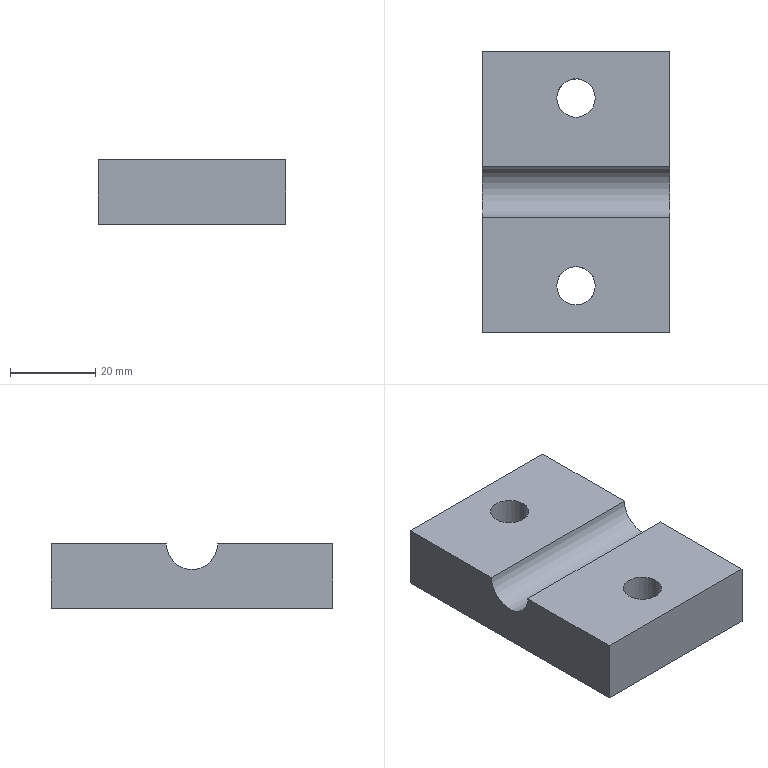Part | 1 solid | 12 faces | box 44 x 66 x 15 mm | volume 39164 mm3 | plane 7 | cylinder 5 | commonest cylinder face diameters 9 x4 12 x1
STEP:
#1=CARTESIAN_POINT('',(0.,0.,0.));
#2=DIRECTION('',(0.,0.,1.));
#3=DIRECTION('',(1.,0.,0.));
#4=AXIS2_PLACEMENT_3D('',#1,#2,#3);
#5=CARTESIAN_POINT('',(-482.433,147.5,-310.6));
#6=VERTEX_POINT('',#5);
#7=CARTESIAN_POINT('',(-526.433,147.5,-310.6));
#8=VERTEX_POINT('',#7);
#9=CARTESIAN_POINT('',(-517.416,147.5,-310.6));
#10=DIRECTION('',(-1.,0.,0.));
#11=VECTOR('',#10,1.);
#12=LINE('',#9,#11);
#13=CARTESIAN_POINT('',(-504.433,141.5,-310.6));
#14=DIRECTION('',(0.,0.,1.));
#15=DIRECTION('',(-1.,0.,0.));
#16=AXIS2_PLACEMENT_3D('',#13,#14,#15);
#17=PLANE('',#16);
#18=CARTESIAN_POINT('',(12.983,-6.));
#19=DIRECTION('',(1.,0.));
#20=VECTOR('',#19,1.);
#21=LINE('',#18,#20);
#22=(GEOMETRIC_REPRESENTATION_CONTEXT(2)PARAMETRIC_REPRESENTATION_CONTEXT()REPRESENTATION_CONTEXT('',''));
#23=DEFINITIONAL_REPRESENTATION('',(#21),#22);
#24=PCURVE('',#17,#23);
#25=CARTESIAN_POINT('',(-517.416,141.5,-310.6));
#26=DIRECTION('',(-1.,0.,0.));
#27=DIRECTION('',(0.,0.,1.));
#28=AXIS2_PLACEMENT_3D('',#25,#26,#27);
#29=CYLINDRICAL_SURFACE('',#28,6.);
#30=CARTESIAN_POINT('',(1.571,0.));
#31=DIRECTION('',(0.,1.));
#32=VECTOR('',#31,1.);
#33=LINE('',#30,#32);
#34=(GEOMETRIC_REPRESENTATION_CONTEXT(2)PARAMETRIC_REPRESENTATION_CONTEXT()REPRESENTATION_CONTEXT('',''));
#35=DEFINITIONAL_REPRESENTATION('',(#33),#34);
#36=PCURVE('',#29,#35);
#37=SURFACE_CURVE('',#12,(#24,#36),.PCURVE_S1.);
#38=EDGE_CURVE('',#6,#8,#37,.T.);
#39=ORIENTED_EDGE('',*,*,#38,.F.);
#40=CARTESIAN_POINT('',(-482.433,174.5,-310.6));
#41=VERTEX_POINT('',#40);
#42=CARTESIAN_POINT('',(-482.433,141.5,-310.6));
#43=DIRECTION('',(0.,-1.,0.));
#44=VECTOR('',#43,1.);
#45=LINE('',#42,#44);
#46=CARTESIAN_POINT('',(-22.,0.));
#47=DIRECTION('',(0.,1.));
#48=VECTOR('',#47,1.);
#49=LINE('',#46,#48);
#50=(GEOMETRIC_REPRESENTATION_CONTEXT(2)PARAMETRIC_REPRESENTATION_CONTEXT()REPRESENTATION_CONTEXT('',''));
#51=DEFINITIONAL_REPRESENTATION('',(#49),#50);
#52=PCURVE('',#17,#51);
#53=CARTESIAN_POINT('',(-482.433,141.5,-319.1));
#54=DIRECTION('',(1.,0.,0.));
#55=DIRECTION('',(0.,0.,1.));
#56=AXIS2_PLACEMENT_3D('',#53,#54,#55);
#57=PLANE('',#56);
#58=CARTESIAN_POINT('',(8.5,0.));
#59=DIRECTION('',(0.,1.));
#60=VECTOR('',#59,1.);
#61=LINE('',#58,#60);
#62=(GEOMETRIC_REPRESENTATION_CONTEXT(2)PARAMETRIC_REPRESENTATION_CONTEXT()REPRESENTATION_CONTEXT('',''));
#63=DEFINITIONAL_REPRESENTATION('',(#61),#62);
#64=PCURVE('',#57,#63);
#65=SURFACE_CURVE('',#45,(#52,#64),.PCURVE_S1.);
#66=EDGE_CURVE('',#41,#6,#65,.T.);
#67=ORIENTED_EDGE('',*,*,#66,.F.);
#68=CARTESIAN_POINT('',(-526.433,174.5,-310.6));
#69=VERTEX_POINT('',#68);
#70=CARTESIAN_POINT('',(-504.433,174.5,-310.6));
#71=DIRECTION('',(1.,0.,0.));
#72=VECTOR('',#71,1.);
#73=LINE('',#70,#72);
#74=CARTESIAN_POINT('',(0.,-33.));
#75=DIRECTION('',(-1.,0.));
#76=VECTOR('',#75,1.);
#77=LINE('',#74,#76);
#78=(GEOMETRIC_REPRESENTATION_CONTEXT(2)PARAMETRIC_REPRESENTATION_CONTEXT()REPRESENTATION_CONTEXT('',''));
#79=DEFINITIONAL_REPRESENTATION('',(#77),#78);
#80=PCURVE('',#17,#79);
#81=CARTESIAN_POINT('',(-504.433,174.5,-319.1));
#82=DIRECTION('',(0.,1.,0.));
#83=DIRECTION('',(0.,0.,-1.));
#84=AXIS2_PLACEMENT_3D('',#81,#82,#83);
#85=PLANE('',#84);
#86=CARTESIAN_POINT('',(-8.5,0.));
#87=DIRECTION('',(0.,-1.));
#88=VECTOR('',#87,1.);
#89=LINE('',#86,#88);
#90=(GEOMETRIC_REPRESENTATION_CONTEXT(2)PARAMETRIC_REPRESENTATION_CONTEXT()REPRESENTATION_CONTEXT('',''));
#91=DEFINITIONAL_REPRESENTATION('',(#89),#90);
#92=PCURVE('',#85,#91);
#93=SURFACE_CURVE('',#73,(#80,#92),.PCURVE_S1.);
#94=EDGE_CURVE('',#69,#41,#93,.T.);
#95=ORIENTED_EDGE('',*,*,#94,.F.);
#96=CARTESIAN_POINT('',(-526.433,141.5,-310.6));
#97=DIRECTION('',(0.,1.,0.));
#98=VECTOR('',#97,1.);
#99=LINE('',#96,#98);
#100=CARTESIAN_POINT('',(22.,0.));
#101=DIRECTION('',(0.,-1.));
#102=VECTOR('',#101,1.);
#103=LINE('',#100,#102);
#104=(GEOMETRIC_REPRESENTATION_CONTEXT(2)PARAMETRIC_REPRESENTATION_CONTEXT()REPRESENTATION_CONTEXT('',''));
#105=DEFINITIONAL_REPRESENTATION('',(#103),#104);
#106=PCURVE('',#17,#105);
#107=CARTESIAN_POINT('',(-526.433,141.5,-319.1));
#108=DIRECTION('',(-1.,0.,0.));
#109=DIRECTION('',(0.,0.,-1.));
#110=AXIS2_PLACEMENT_3D('',#107,#108,#109);
#111=PLANE('',#110);
#112=CARTESIAN_POINT('',(-8.5,0.));
#113=DIRECTION('',(0.,-1.));
#114=VECTOR('',#113,1.);
#115=LINE('',#112,#114);
#116=(GEOMETRIC_REPRESENTATION_CONTEXT(2)PARAMETRIC_REPRESENTATION_CONTEXT()REPRESENTATION_CONTEXT('',''));
#117=DEFINITIONAL_REPRESENTATION('',(#115),#116);
#118=PCURVE('',#111,#117);
#119=SURFACE_CURVE('',#99,(#106,#118),.PCURVE_S1.);
#120=EDGE_CURVE('',#8,#69,#119,.T.);
#121=ORIENTED_EDGE('',*,*,#120,.F.);
#122=EDGE_LOOP('',(#39,#67,#95,#121));
#123=FACE_BOUND('',#122,.T.);
#124=CARTESIAN_POINT('',(-508.933,163.5,-310.6));
#125=VERTEX_POINT('',#124);
#126=CARTESIAN_POINT('',(-499.933,163.5,-310.6));
#127=VERTEX_POINT('',#126);
#128=CARTESIAN_POINT('',(-504.433,163.5,-310.6));
#129=DIRECTION('',(0.,0.,-1.));
#130=DIRECTION('',(-1.,0.,0.));
#131=AXIS2_PLACEMENT_3D('',#128,#129,#130);
#132=CIRCLE('',#131,4.5);
#133=CARTESIAN_POINT('',(4.5,-22.));
#134=CARTESIAN_POINT('',(4.5,-29.794));
#135=CARTESIAN_POINT('',(-2.25,-25.897));
#136=CARTESIAN_POINT('',(-9.,-22.));
#137=CARTESIAN_POINT('',(-2.25,-18.103));
#138=CARTESIAN_POINT('',(4.5,-14.206));
#139=CARTESIAN_POINT('',(4.5,-22.));
#140=(BOUNDED_CURVE()B_SPLINE_CURVE(2,(#133,#134,#135,#136,#137,#138,#139),.UNSPECIFIED.,.T.,.F.)B_SPLINE_CURVE_WITH_KNOTS((1,2,2,2,2,1),(-2.094,0.,2.094,4.189,6.283,8.378),.UNSPECIFIED.)CURVE()GEOMETRIC_REPRESENTATION_ITEM()RATIONAL_B_SPLINE_CURVE((1.,0.5,1.,0.5,1.,0.5,1.))REPRESENTATION_ITEM(''));
#141=(GEOMETRIC_REPRESENTATION_CONTEXT(2)PARAMETRIC_REPRESENTATION_CONTEXT()REPRESENTATION_CONTEXT('',''));
#142=DEFINITIONAL_REPRESENTATION('',(#140),#141);
#143=PCURVE('',#17,#142);
#144=CARTESIAN_POINT('',(-504.433,163.5,-608.599));
#145=DIRECTION('',(0.,0.,1.));
#146=DIRECTION('',(0.,-1.,0.));
#147=AXIS2_PLACEMENT_3D('',#144,#145,#146);
#148=CYLINDRICAL_SURFACE('',#147,4.5);
#149=CARTESIAN_POINT('',(4.712,297.999));
#150=DIRECTION('',(-1.,0.));
#151=VECTOR('',#150,1.);
#152=LINE('',#149,#151);
#153=(GEOMETRIC_REPRESENTATION_CONTEXT(2)PARAMETRIC_REPRESENTATION_CONTEXT()REPRESENTATION_CONTEXT('',''));
#154=DEFINITIONAL_REPRESENTATION('',(#152),#153);
#155=PCURVE('',#148,#154);
#156=SURFACE_CURVE('',#132,(#143,#155),.PCURVE_S1.);
#157=EDGE_CURVE('',#125,#127,#156,.T.);
#158=ORIENTED_EDGE('',*,*,#157,.T.);
#159=CARTESIAN_POINT('',(-504.433,163.5,-310.6));
#160=DIRECTION('',(0.,0.,-1.));
#161=DIRECTION('',(-1.,0.,0.));
#162=AXIS2_PLACEMENT_3D('',#159,#160,#161);
#163=CIRCLE('',#162,4.5);
#164=CARTESIAN_POINT('',(4.5,-22.));
#165=CARTESIAN_POINT('',(4.5,-29.794));
#166=CARTESIAN_POINT('',(-2.25,-25.897));
#167=CARTESIAN_POINT('',(-9.,-22.));
#168=CARTESIAN_POINT('',(-2.25,-18.103));
#169=CARTESIAN_POINT('',(4.5,-14.206));
#170=CARTESIAN_POINT('',(4.5,-22.));
#171=(BOUNDED_CURVE()B_SPLINE_CURVE(2,(#164,#165,#166,#167,#168,#169,#170),.UNSPECIFIED.,.T.,.F.)B_SPLINE_CURVE_WITH_KNOTS((1,2,2,2,2,1),(-2.094,0.,2.094,4.189,6.283,8.378),.UNSPECIFIED.)CURVE()GEOMETRIC_REPRESENTATION_ITEM()RATIONAL_B_SPLINE_CURVE((1.,0.5,1.,0.5,1.,0.5,1.))REPRESENTATION_ITEM(''));
#172=(GEOMETRIC_REPRESENTATION_CONTEXT(2)PARAMETRIC_REPRESENTATION_CONTEXT()REPRESENTATION_CONTEXT('',''));
#173=DEFINITIONAL_REPRESENTATION('',(#171),#172);
#174=PCURVE('',#17,#173);
#175=CARTESIAN_POINT('',(-504.433,163.5,-608.599));
#176=DIRECTION('',(0.,0.,1.));
#177=DIRECTION('',(0.,1.,0.));
#178=AXIS2_PLACEMENT_3D('',#175,#176,#177);
#179=CYLINDRICAL_SURFACE('',#178,4.5);
#180=CARTESIAN_POINT('',(7.854,297.999));
#181=DIRECTION('',(-1.,0.));
#182=VECTOR('',#181,1.);
#183=LINE('',#180,#182);
#184=(GEOMETRIC_REPRESENTATION_CONTEXT(2)PARAMETRIC_REPRESENTATION_CONTEXT()REPRESENTATION_CONTEXT('',''));
#185=DEFINITIONAL_REPRESENTATION('',(#183),#184);
#186=PCURVE('',#179,#185);
#187=SURFACE_CURVE('',#163,(#174,#186),.PCURVE_S1.);
#188=EDGE_CURVE('',#127,#125,#187,.T.);
#189=ORIENTED_EDGE('',*,*,#188,.T.);
#190=EDGE_LOOP('',(#158,#189));
#191=FACE_BOUND('',#190,.T.);
#192=ADVANCED_FACE('',(#123,#191),#17,.T.);
#193=CARTESIAN_POINT('',(-499.933,163.5,-325.6));
#194=VERTEX_POINT('',#193);
#195=CARTESIAN_POINT('',(-508.933,163.5,-325.6));
#196=VERTEX_POINT('',#195);
#197=CARTESIAN_POINT('',(-499.933,163.5,-325.6));
#198=CARTESIAN_POINT('',(-499.933,164.914,-325.6));
#199=CARTESIAN_POINT('',(-500.486,166.328,-325.6));
#200=CARTESIAN_POINT('',(-501.604,167.447,-325.6));
#201=CARTESIAN_POINT('',(-504.433,168.554,-325.6));
#202=CARTESIAN_POINT('',(-507.261,167.446,-325.6));
#203=CARTESIAN_POINT('',(-508.38,166.329,-325.6));
#204=CARTESIAN_POINT('',(-508.933,164.913,-325.6));
#205=CARTESIAN_POINT('',(-508.933,163.5,-325.6));
#206=B_SPLINE_CURVE_WITH_KNOTS('',5,(#197,#198,#199,#200,#201,#202,#203,#204,#205),.UNSPECIFIED.,.F.,.F.,(6,3,6),(3.142,4.712,6.283),.UNSPECIFIED.);
#207=CARTESIAN_POINT('',(-1.571,282.999));
#208=DIRECTION('',(1.,0.));
#209=VECTOR('',#208,1.);
#210=LINE('',#207,#209);
#211=(GEOMETRIC_REPRESENTATION_CONTEXT(2)PARAMETRIC_REPRESENTATION_CONTEXT()REPRESENTATION_CONTEXT('',''));
#212=DEFINITIONAL_REPRESENTATION('',(#210),#211);
#213=PCURVE('',#148,#212);
#214=CARTESIAN_POINT('',(-492.022,-194.5,-325.6));
#215=DIRECTION('',(-0.00001444,0.,-1.));
#216=DIRECTION('',(1.,0.,-0.00001444));
#217=AXIS2_PLACEMENT_3D('',#214,#215,#216);
#218=PLANE('',#217);
#219=CARTESIAN_POINT('',(-7.911,-358.));
#220=CARTESIAN_POINT('',(-7.911,-359.414));
#221=CARTESIAN_POINT('',(-8.464,-360.828));
#222=CARTESIAN_POINT('',(-9.582,-361.946));
#223=CARTESIAN_POINT('',(-12.411,-363.053));
#224=CARTESIAN_POINT('',(-15.239,-361.946));
#225=CARTESIAN_POINT('',(-16.358,-360.829));
#226=CARTESIAN_POINT('',(-16.911,-359.413));
#227=CARTESIAN_POINT('',(-16.911,-358.));
#228=B_SPLINE_CURVE_WITH_KNOTS('',5,(#219,#220,#221,#222,#223,#224,#225,#226,#227),.UNSPECIFIED.,.F.,.F.,(6,3,6),(3.142,4.712,6.283),.UNSPECIFIED.);
#229=(GEOMETRIC_REPRESENTATION_CONTEXT(2)PARAMETRIC_REPRESENTATION_CONTEXT()REPRESENTATION_CONTEXT('',''));
#230=DEFINITIONAL_REPRESENTATION('',(#228),#229);
#231=PCURVE('',#218,#230);
#232=SURFACE_CURVE('',#206,(#213,#231),.PCURVE_S1.);
#233=EDGE_CURVE('',#194,#196,#232,.T.);
#234=ORIENTED_EDGE('',*,*,#233,.T.);
#235=CARTESIAN_POINT('',(-508.933,163.5,-325.6));
#236=DIRECTION('',(0.,0.,1.));
#237=VECTOR('',#236,1.);
#238=LINE('',#235,#237);
#239=CARTESIAN_POINT('',(4.712,282.999));
#240=DIRECTION('',(0.,1.));
#241=VECTOR('',#240,1.);
#242=LINE('',#239,#241);
#243=(GEOMETRIC_REPRESENTATION_CONTEXT(2)PARAMETRIC_REPRESENTATION_CONTEXT()REPRESENTATION_CONTEXT('',''));
#244=DEFINITIONAL_REPRESENTATION('',(#242),#243);
#245=PCURVE('',#148,#244);
#246=CARTESIAN_POINT('',(1.571,282.999));
#247=DIRECTION('',(0.,1.));
#248=VECTOR('',#247,1.);
#249=LINE('',#246,#248);
#250=(GEOMETRIC_REPRESENTATION_CONTEXT(2)PARAMETRIC_REPRESENTATION_CONTEXT()REPRESENTATION_CONTEXT('',''));
#251=DEFINITIONAL_REPRESENTATION('',(#249),#250);
#252=PCURVE('',#179,#251);
#253=SURFACE_CURVE('',#238,(#245,#252),.PCURVE_S1.);
#254=EDGE_CURVE('',#196,#125,#253,.T.);
#255=ORIENTED_EDGE('',*,*,#254,.T.);
#256=ORIENTED_EDGE('',*,*,#157,.T.);
#257=CARTESIAN_POINT('',(-499.933,163.5,-325.6));
#258=DIRECTION('',(0.,0.,1.));
#259=VECTOR('',#258,1.);
#260=LINE('',#257,#259);
#261=CARTESIAN_POINT('',(1.571,282.999));
#262=DIRECTION('',(0.,1.));
#263=VECTOR('',#262,1.);
#264=LINE('',#261,#263);
#265=(GEOMETRIC_REPRESENTATION_CONTEXT(2)PARAMETRIC_REPRESENTATION_CONTEXT()REPRESENTATION_CONTEXT('',''));
#266=DEFINITIONAL_REPRESENTATION('',(#264),#265);
#267=PCURVE('',#148,#266);
#268=CARTESIAN_POINT('',(4.712,282.999));
#269=DIRECTION('',(0.,1.));
#270=VECTOR('',#269,1.);
#271=LINE('',#268,#270);
#272=(GEOMETRIC_REPRESENTATION_CONTEXT(2)PARAMETRIC_REPRESENTATION_CONTEXT()REPRESENTATION_CONTEXT('',''));
#273=DEFINITIONAL_REPRESENTATION('',(#271),#272);
#274=PCURVE('',#179,#273);
#275=SURFACE_CURVE('',#260,(#267,#274),.PCURVE_S1.);
#276=EDGE_CURVE('',#194,#127,#275,.T.);
#277=ORIENTED_EDGE('',*,*,#276,.F.);
#278=EDGE_LOOP('',(#234,#255,#256,#277));
#279=FACE_BOUND('',#278,.F.);
#280=ADVANCED_FACE('',(#279),#148,.F.);
#281=CARTESIAN_POINT('',(-508.933,119.5,-325.6));
#282=VERTEX_POINT('',#281);
#283=CARTESIAN_POINT('',(-499.933,119.5,-325.6));
#284=VERTEX_POINT('',#283);
#285=CARTESIAN_POINT('',(-508.933,119.5,-325.6));
#286=CARTESIAN_POINT('',(-508.933,118.087,-325.6));
#287=CARTESIAN_POINT('',(-508.38,116.671,-325.6));
#288=CARTESIAN_POINT('',(-507.261,115.554,-325.6));
#289=CARTESIAN_POINT('',(-504.433,114.446,-325.6));
#290=CARTESIAN_POINT('',(-501.604,115.554,-325.6));
#291=CARTESIAN_POINT('',(-500.486,116.672,-325.6));
#292=CARTESIAN_POINT('',(-499.933,118.086,-325.6));
#293=CARTESIAN_POINT('',(-499.933,119.5,-325.6));
#294=B_SPLINE_CURVE_WITH_KNOTS('',5,(#285,#286,#287,#288,#289,#290,#291,#292,#293),.UNSPECIFIED.,.F.,.F.,(6,3,6),(0.,1.571,3.142),.UNSPECIFIED.);
#295=CARTESIAN_POINT('',(-16.911,-314.));
#296=CARTESIAN_POINT('',(-16.911,-312.587));
#297=CARTESIAN_POINT('',(-16.358,-311.171));
#298=CARTESIAN_POINT('',(-15.239,-310.054));
#299=CARTESIAN_POINT('',(-12.411,-308.946));
#300=CARTESIAN_POINT('',(-9.582,-310.053));
#301=CARTESIAN_POINT('',(-8.464,-311.172));
#302=CARTESIAN_POINT('',(-7.911,-312.586));
#303=CARTESIAN_POINT('',(-7.911,-314.));
#304=B_SPLINE_CURVE_WITH_KNOTS('',5,(#295,#296,#297,#298,#299,#300,#301,#302,#303),.UNSPECIFIED.,.F.,.F.,(6,3,6),(0.,1.571,3.142),.UNSPECIFIED.);
#305=(GEOMETRIC_REPRESENTATION_CONTEXT(2)PARAMETRIC_REPRESENTATION_CONTEXT()REPRESENTATION_CONTEXT('',''));
#306=DEFINITIONAL_REPRESENTATION('',(#304),#305);
#307=PCURVE('',#218,#306);
#308=CARTESIAN_POINT('',(-504.433,119.5,-608.599));
#309=DIRECTION('',(0.,0.,1.));
#310=DIRECTION('',(0.,1.,0.));
#311=AXIS2_PLACEMENT_3D('',#308,#309,#310);
#312=CYLINDRICAL_SURFACE('',#311,4.5);
#313=CARTESIAN_POINT('',(1.571,282.999));
#314=DIRECTION('',(1.,0.));
#315=VECTOR('',#314,1.);
#316=LINE('',#313,#315);
#317=(GEOMETRIC_REPRESENTATION_CONTEXT(2)PARAMETRIC_REPRESENTATION_CONTEXT()REPRESENTATION_CONTEXT('',''));
#318=DEFINITIONAL_REPRESENTATION('',(#316),#317);
#319=PCURVE('',#312,#318);
#320=SURFACE_CURVE('',#294,(#307,#319),.PCURVE_S1.);
#321=EDGE_CURVE('',#282,#284,#320,.T.);
#322=ORIENTED_EDGE('',*,*,#321,.T.);
#323=CARTESIAN_POINT('',(-499.933,119.5,-325.6));
#324=CARTESIAN_POINT('',(-499.933,120.914,-325.6));
#325=CARTESIAN_POINT('',(-500.486,122.328,-325.6));
#326=CARTESIAN_POINT('',(-501.604,123.447,-325.6));
#327=CARTESIAN_POINT('',(-504.433,124.554,-325.6));
#328=CARTESIAN_POINT('',(-507.261,123.446,-325.6));
#329=CARTESIAN_POINT('',(-508.38,122.329,-325.6));
#330=CARTESIAN_POINT('',(-508.933,120.913,-325.6));
#331=CARTESIAN_POINT('',(-508.933,119.5,-325.6));
#332=B_SPLINE_CURVE_WITH_KNOTS('',5,(#323,#324,#325,#326,#327,#328,#329,#330,#331),.UNSPECIFIED.,.F.,.F.,(6,3,6),(3.142,4.712,6.283),.UNSPECIFIED.);
#333=CARTESIAN_POINT('',(-7.911,-314.));
#334=CARTESIAN_POINT('',(-7.911,-315.414));
#335=CARTESIAN_POINT('',(-8.464,-316.828));
#336=CARTESIAN_POINT('',(-9.582,-317.946));
#337=CARTESIAN_POINT('',(-12.411,-319.053));
#338=CARTESIAN_POINT('',(-15.239,-317.946));
#339=CARTESIAN_POINT('',(-16.358,-316.829));
#340=CARTESIAN_POINT('',(-16.911,-315.413));
#341=CARTESIAN_POINT('',(-16.911,-314.));
#342=B_SPLINE_CURVE_WITH_KNOTS('',5,(#333,#334,#335,#336,#337,#338,#339,#340,#341),.UNSPECIFIED.,.F.,.F.,(6,3,6),(3.142,4.712,6.283),.UNSPECIFIED.);
#343=(GEOMETRIC_REPRESENTATION_CONTEXT(2)PARAMETRIC_REPRESENTATION_CONTEXT()REPRESENTATION_CONTEXT('',''));
#344=DEFINITIONAL_REPRESENTATION('',(#342),#343);
#345=PCURVE('',#218,#344);
#346=CARTESIAN_POINT('',(-504.433,119.5,-608.599));
#347=DIRECTION('',(0.,0.,1.));
#348=DIRECTION('',(0.,-1.,0.));
#349=AXIS2_PLACEMENT_3D('',#346,#347,#348);
#350=CYLINDRICAL_SURFACE('',#349,4.5);
#351=CARTESIAN_POINT('',(-1.571,282.999));
#352=DIRECTION('',(1.,0.));
#353=VECTOR('',#352,1.);
#354=LINE('',#351,#353);
#355=(GEOMETRIC_REPRESENTATION_CONTEXT(2)PARAMETRIC_REPRESENTATION_CONTEXT()REPRESENTATION_CONTEXT('',''));
#356=DEFINITIONAL_REPRESENTATION('',(#354),#355);
#357=PCURVE('',#350,#356);
#358=SURFACE_CURVE('',#332,(#345,#357),.PCURVE_S1.);
#359=EDGE_CURVE('',#284,#282,#358,.T.);
#360=ORIENTED_EDGE('',*,*,#359,.T.);
#361=EDGE_LOOP('',(#322,#360));
#362=FACE_BOUND('',#361,.T.);
#363=CARTESIAN_POINT('',(-482.433,108.5,-325.6));
#364=VERTEX_POINT('',#363);
#365=CARTESIAN_POINT('',(-482.433,174.5,-325.6));
#366=VERTEX_POINT('',#365);
#367=CARTESIAN_POINT('',(-482.433,141.5,-325.6));
#368=DIRECTION('',(0.,1.,0.));
#369=VECTOR('',#368,1.);
#370=LINE('',#367,#369);
#371=CARTESIAN_POINT('',(9.589,-336.));
#372=DIRECTION('',(0.,-1.));
#373=VECTOR('',#372,1.);
#374=LINE('',#371,#373);
#375=(GEOMETRIC_REPRESENTATION_CONTEXT(2)PARAMETRIC_REPRESENTATION_CONTEXT()REPRESENTATION_CONTEXT('',''));
#376=DEFINITIONAL_REPRESENTATION('',(#374),#375);
#377=PCURVE('',#218,#376);
#378=CARTESIAN_POINT('',(-6.5,0.));
#379=DIRECTION('',(0.,-1.));
#380=VECTOR('',#379,1.);
#381=LINE('',#378,#380);
#382=(GEOMETRIC_REPRESENTATION_CONTEXT(2)PARAMETRIC_REPRESENTATION_CONTEXT()REPRESENTATION_CONTEXT('',''));
#383=DEFINITIONAL_REPRESENTATION('',(#381),#382);
#384=PCURVE('',#57,#383);
#385=SURFACE_CURVE('',#370,(#377,#384),.PCURVE_S1.);
#386=EDGE_CURVE('',#364,#366,#385,.T.);
#387=ORIENTED_EDGE('',*,*,#386,.F.);
#388=CARTESIAN_POINT('',(-526.433,108.5,-325.6));
#389=VERTEX_POINT('',#388);
#390=CARTESIAN_POINT('',(-504.433,108.5,-325.6));
#391=DIRECTION('',(1.,0.,-0.00001444));
#392=VECTOR('',#391,1.);
#393=LINE('',#390,#392);
#394=CARTESIAN_POINT('',(-12.411,-303.));
#395=DIRECTION('',(1.,0.));
#396=VECTOR('',#395,1.);
#397=LINE('',#394,#396);
#398=(GEOMETRIC_REPRESENTATION_CONTEXT(2)PARAMETRIC_REPRESENTATION_CONTEXT()REPRESENTATION_CONTEXT('',''));
#399=DEFINITIONAL_REPRESENTATION('',(#397),#398);
#400=PCURVE('',#218,#399);
#401=CARTESIAN_POINT('',(-504.433,108.5,-319.1));
#402=DIRECTION('',(0.,-1.,0.));
#403=DIRECTION('',(0.,0.,1.));
#404=AXIS2_PLACEMENT_3D('',#401,#402,#403);
#405=PLANE('',#404);
#406=CARTESIAN_POINT('',(-6.5,0.00009388));
#407=DIRECTION('',(-0.00001444,-1.));
#408=VECTOR('',#407,1.);
#409=LINE('',#406,#408);
#410=(GEOMETRIC_REPRESENTATION_CONTEXT(2)PARAMETRIC_REPRESENTATION_CONTEXT()REPRESENTATION_CONTEXT('',''));
#411=DEFINITIONAL_REPRESENTATION('',(#409),#410);
#412=PCURVE('',#405,#411);
#413=SURFACE_CURVE('',#393,(#400,#412),.PCURVE_S1.);
#414=EDGE_CURVE('',#389,#364,#413,.T.);
#415=ORIENTED_EDGE('',*,*,#414,.F.);
#416=CARTESIAN_POINT('',(-526.433,174.5,-325.6));
#417=VERTEX_POINT('',#416);
#418=CARTESIAN_POINT('',(-526.433,141.5,-325.6));
#419=DIRECTION('',(0.,-1.,0.));
#420=VECTOR('',#419,1.);
#421=LINE('',#418,#420);
#422=CARTESIAN_POINT('',(-34.411,-336.));
#423=DIRECTION('',(0.,1.));
#424=VECTOR('',#423,1.);
#425=LINE('',#422,#424);
#426=(GEOMETRIC_REPRESENTATION_CONTEXT(2)PARAMETRIC_REPRESENTATION_CONTEXT()REPRESENTATION_CONTEXT('',''));
#427=DEFINITIONAL_REPRESENTATION('',(#425),#426);
#428=PCURVE('',#218,#427);
#429=CARTESIAN_POINT('',(6.5,0.));
#430=DIRECTION('',(0.,1.));
#431=VECTOR('',#430,1.);
#432=LINE('',#429,#431);
#433=(GEOMETRIC_REPRESENTATION_CONTEXT(2)PARAMETRIC_REPRESENTATION_CONTEXT()REPRESENTATION_CONTEXT('',''));
#434=DEFINITIONAL_REPRESENTATION('',(#432),#433);
#435=PCURVE('',#111,#434);
#436=SURFACE_CURVE('',#421,(#428,#435),.PCURVE_S1.);
#437=EDGE_CURVE('',#417,#389,#436,.T.);
#438=ORIENTED_EDGE('',*,*,#437,.F.);
#439=CARTESIAN_POINT('',(-504.433,174.5,-325.6));
#440=DIRECTION('',(-1.,0.,0.00001444));
#441=VECTOR('',#440,1.);
#442=LINE('',#439,#441);
#443=CARTESIAN_POINT('',(-12.411,-369.));
#444=DIRECTION('',(-1.,0.));
#445=VECTOR('',#444,1.);
#446=LINE('',#443,#445);
#447=(GEOMETRIC_REPRESENTATION_CONTEXT(2)PARAMETRIC_REPRESENTATION_CONTEXT()REPRESENTATION_CONTEXT('',''));
#448=DEFINITIONAL_REPRESENTATION('',(#446),#447);
#449=PCURVE('',#218,#448);
#450=CARTESIAN_POINT('',(6.5,0.00009388));
#451=DIRECTION('',(-0.00001444,1.));
#452=VECTOR('',#451,1.);
#453=LINE('',#450,#452);
#454=(GEOMETRIC_REPRESENTATION_CONTEXT(2)PARAMETRIC_REPRESENTATION_CONTEXT()REPRESENTATION_CONTEXT('',''));
#455=DEFINITIONAL_REPRESENTATION('',(#453),#454);
#456=PCURVE('',#85,#455);
#457=SURFACE_CURVE('',#442,(#449,#456),.PCURVE_S1.);
#458=EDGE_CURVE('',#366,#417,#457,.T.);
#459=ORIENTED_EDGE('',*,*,#458,.F.);
#460=EDGE_LOOP('',(#387,#415,#438,#459));
#461=FACE_BOUND('',#460,.T.);
#462=CARTESIAN_POINT('',(-508.933,163.5,-325.6));
#463=CARTESIAN_POINT('',(-508.933,162.087,-325.6));
#464=CARTESIAN_POINT('',(-508.38,160.671,-325.6));
#465=CARTESIAN_POINT('',(-507.261,159.554,-325.6));
#466=CARTESIAN_POINT('',(-504.433,158.446,-325.6));
#467=CARTESIAN_POINT('',(-501.604,159.554,-325.6));
#468=CARTESIAN_POINT('',(-500.486,160.672,-325.6));
#469=CARTESIAN_POINT('',(-499.933,162.086,-325.6));
#470=CARTESIAN_POINT('',(-499.933,163.5,-325.6));
#471=B_SPLINE_CURVE_WITH_KNOTS('',5,(#462,#463,#464,#465,#466,#467,#468,#469,#470),.UNSPECIFIED.,.F.,.F.,(6,3,6),(0.,1.571,3.142),.UNSPECIFIED.);
#472=CARTESIAN_POINT('',(-16.911,-358.));
#473=CARTESIAN_POINT('',(-16.911,-356.587));
#474=CARTESIAN_POINT('',(-16.358,-355.171));
#475=CARTESIAN_POINT('',(-15.239,-354.054));
#476=CARTESIAN_POINT('',(-12.411,-352.946));
#477=CARTESIAN_POINT('',(-9.582,-354.053));
#478=CARTESIAN_POINT('',(-8.464,-355.172));
#479=CARTESIAN_POINT('',(-7.911,-356.586));
#480=CARTESIAN_POINT('',(-7.911,-358.));
#481=B_SPLINE_CURVE_WITH_KNOTS('',5,(#472,#473,#474,#475,#476,#477,#478,#479,#480),.UNSPECIFIED.,.F.,.F.,(6,3,6),(0.,1.571,3.142),.UNSPECIFIED.);
#482=(GEOMETRIC_REPRESENTATION_CONTEXT(2)PARAMETRIC_REPRESENTATION_CONTEXT()REPRESENTATION_CONTEXT('',''));
#483=DEFINITIONAL_REPRESENTATION('',(#481),#482);
#484=PCURVE('',#218,#483);
#485=CARTESIAN_POINT('',(1.571,282.999));
#486=DIRECTION('',(1.,0.));
#487=VECTOR('',#486,1.);
#488=LINE('',#485,#487);
#489=(GEOMETRIC_REPRESENTATION_CONTEXT(2)PARAMETRIC_REPRESENTATION_CONTEXT()REPRESENTATION_CONTEXT('',''));
#490=DEFINITIONAL_REPRESENTATION('',(#488),#489);
#491=PCURVE('',#179,#490);
#492=SURFACE_CURVE('',#471,(#484,#491),.PCURVE_S1.);
#493=EDGE_CURVE('',#196,#194,#492,.T.);
#494=ORIENTED_EDGE('',*,*,#493,.T.);
#495=ORIENTED_EDGE('',*,*,#233,.T.);
#496=EDGE_LOOP('',(#494,#495));
#497=FACE_BOUND('',#496,.T.);
#498=ADVANCED_FACE('',(#362,#461,#497),#218,.T.);
#499=CARTESIAN_POINT('',(-526.433,174.5,-319.1));
#500=DIRECTION('',(0.,0.,1.));
#501=VECTOR('',#500,1.);
#502=LINE('',#499,#501);
#503=CARTESIAN_POINT('',(0.,22.));
#504=DIRECTION('',(-1.,0.));
#505=VECTOR('',#504,1.);
#506=LINE('',#503,#505);
#507=(GEOMETRIC_REPRESENTATION_CONTEXT(2)PARAMETRIC_REPRESENTATION_CONTEXT()REPRESENTATION_CONTEXT('',''));
#508=DEFINITIONAL_REPRESENTATION('',(#506),#507);
#509=PCURVE('',#85,#508);
#510=CARTESIAN_POINT('',(0.,-33.));
#511=DIRECTION('',(-1.,0.));
#512=VECTOR('',#511,1.);
#513=LINE('',#510,#512);
#514=(GEOMETRIC_REPRESENTATION_CONTEXT(2)PARAMETRIC_REPRESENTATION_CONTEXT()REPRESENTATION_CONTEXT('',''));
#515=DEFINITIONAL_REPRESENTATION('',(#513),#514);
#516=PCURVE('',#111,#515);
#517=SURFACE_CURVE('',#502,(#509,#516),.PCURVE_S1.);
#518=EDGE_CURVE('',#417,#69,#517,.T.);
#519=ORIENTED_EDGE('',*,*,#518,.T.);
#520=ORIENTED_EDGE('',*,*,#94,.T.);
#521=CARTESIAN_POINT('',(-482.433,174.5,-319.1));
#522=DIRECTION('',(0.,0.,1.));
#523=VECTOR('',#522,1.);
#524=LINE('',#521,#523);
#525=CARTESIAN_POINT('',(0.,-22.));
#526=DIRECTION('',(-1.,0.));
#527=VECTOR('',#526,1.);
#528=LINE('',#525,#527);
#529=(GEOMETRIC_REPRESENTATION_CONTEXT(2)PARAMETRIC_REPRESENTATION_CONTEXT()REPRESENTATION_CONTEXT('',''));
#530=DEFINITIONAL_REPRESENTATION('',(#528),#529);
#531=PCURVE('',#85,#530);
#532=CARTESIAN_POINT('',(0.,-33.));
#533=DIRECTION('',(1.,0.));
#534=VECTOR('',#533,1.);
#535=LINE('',#532,#534);
#536=(GEOMETRIC_REPRESENTATION_CONTEXT(2)PARAMETRIC_REPRESENTATION_CONTEXT()REPRESENTATION_CONTEXT('',''));
#537=DEFINITIONAL_REPRESENTATION('',(#535),#536);
#538=PCURVE('',#57,#537);
#539=SURFACE_CURVE('',#524,(#531,#538),.PCURVE_S1.);
#540=EDGE_CURVE('',#366,#41,#539,.T.);
#541=ORIENTED_EDGE('',*,*,#540,.F.);
#542=ORIENTED_EDGE('',*,*,#458,.T.);
#543=EDGE_LOOP('',(#519,#520,#541,#542));
#544=FACE_BOUND('',#543,.T.);
#545=ADVANCED_FACE('',(#544),#85,.T.);
#546=ORIENTED_EDGE('',*,*,#66,.T.);
#547=CARTESIAN_POINT('',(-482.433,135.5,-310.6));
#548=VERTEX_POINT('',#547);
#549=CARTESIAN_POINT('',(-482.433,141.5,-310.6));
#550=DIRECTION('',(1.,0.,0.));
#551=DIRECTION('',(0.,0.,-1.));
#552=AXIS2_PLACEMENT_3D('',#549,#550,#551);
#553=CIRCLE('',#552,6.);
#554=CARTESIAN_POINT('',(8.5,0.));
#555=DIRECTION('',(-1.,0.));
#556=AXIS2_PLACEMENT_2D('',#554,#555);
#557=CIRCLE('',#556,6.);
#558=(GEOMETRIC_REPRESENTATION_CONTEXT(2)PARAMETRIC_REPRESENTATION_CONTEXT()REPRESENTATION_CONTEXT('',''));
#559=DEFINITIONAL_REPRESENTATION('',(#557),#558);
#560=PCURVE('',#57,#559);
#561=CARTESIAN_POINT('',(9.425,-34.983));
#562=DIRECTION('',(-1.,0.));
#563=VECTOR('',#562,1.);
#564=LINE('',#561,#563);
#565=(GEOMETRIC_REPRESENTATION_CONTEXT(2)PARAMETRIC_REPRESENTATION_CONTEXT()REPRESENTATION_CONTEXT('',''));
#566=DEFINITIONAL_REPRESENTATION('',(#564),#565);
#567=PCURVE('',#29,#566);
#568=SURFACE_CURVE('',#553,(#560,#567),.PCURVE_S1.);
#569=EDGE_CURVE('',#548,#6,#568,.T.);
#570=ORIENTED_EDGE('',*,*,#569,.F.);
#571=CARTESIAN_POINT('',(-482.433,108.5,-310.6));
#572=VERTEX_POINT('',#571);
#573=CARTESIAN_POINT('',(-482.433,141.5,-310.6));
#574=DIRECTION('',(0.,-1.,0.));
#575=VECTOR('',#574,1.);
#576=LINE('',#573,#575);
#577=CARTESIAN_POINT('',(8.5,0.));
#578=DIRECTION('',(0.,1.));
#579=VECTOR('',#578,1.);
#580=LINE('',#577,#579);
#581=(GEOMETRIC_REPRESENTATION_CONTEXT(2)PARAMETRIC_REPRESENTATION_CONTEXT()REPRESENTATION_CONTEXT('',''));
#582=DEFINITIONAL_REPRESENTATION('',(#580),#581);
#583=PCURVE('',#57,#582);
#584=CARTESIAN_POINT('',(-504.433,141.5,-310.6));
#585=DIRECTION('',(0.,0.,1.));
#586=DIRECTION('',(-1.,0.,0.));
#587=AXIS2_PLACEMENT_3D('',#584,#585,#586);
#588=PLANE('',#587);
#589=CARTESIAN_POINT('',(-22.,0.));
#590=DIRECTION('',(0.,1.));
#591=VECTOR('',#590,1.);
#592=LINE('',#589,#591);
#593=(GEOMETRIC_REPRESENTATION_CONTEXT(2)PARAMETRIC_REPRESENTATION_CONTEXT()REPRESENTATION_CONTEXT('',''));
#594=DEFINITIONAL_REPRESENTATION('',(#592),#593);
#595=PCURVE('',#588,#594);
#596=SURFACE_CURVE('',#576,(#583,#595),.PCURVE_S1.);
#597=EDGE_CURVE('',#548,#572,#596,.T.);
#598=ORIENTED_EDGE('',*,*,#597,.T.);
#599=CARTESIAN_POINT('',(-482.433,108.5,-319.1));
#600=DIRECTION('',(0.,0.,1.));
#601=VECTOR('',#600,1.);
#602=LINE('',#599,#601);
#603=CARTESIAN_POINT('',(0.,33.));
#604=DIRECTION('',(1.,0.));
#605=VECTOR('',#604,1.);
#606=LINE('',#603,#605);
#607=(GEOMETRIC_REPRESENTATION_CONTEXT(2)PARAMETRIC_REPRESENTATION_CONTEXT()REPRESENTATION_CONTEXT('',''));
#608=DEFINITIONAL_REPRESENTATION('',(#606),#607);
#609=PCURVE('',#57,#608);
#610=CARTESIAN_POINT('',(0.,-22.));
#611=DIRECTION('',(1.,0.));
#612=VECTOR('',#611,1.);
#613=LINE('',#610,#612);
#614=(GEOMETRIC_REPRESENTATION_CONTEXT(2)PARAMETRIC_REPRESENTATION_CONTEXT()REPRESENTATION_CONTEXT('',''));
#615=DEFINITIONAL_REPRESENTATION('',(#613),#614);
#616=PCURVE('',#405,#615);
#617=SURFACE_CURVE('',#602,(#609,#616),.PCURVE_S1.);
#618=EDGE_CURVE('',#364,#572,#617,.T.);
#619=ORIENTED_EDGE('',*,*,#618,.F.);
#620=ORIENTED_EDGE('',*,*,#386,.T.);
#621=ORIENTED_EDGE('',*,*,#540,.T.);
#622=EDGE_LOOP('',(#546,#570,#598,#619,#620,#621));
#623=FACE_BOUND('',#622,.T.);
#624=ADVANCED_FACE('',(#623),#57,.T.);
#625=ORIENTED_EDGE('',*,*,#618,.T.);
#626=CARTESIAN_POINT('',(-526.433,108.5,-310.6));
#627=VERTEX_POINT('',#626);
#628=CARTESIAN_POINT('',(-504.433,108.5,-310.6));
#629=DIRECTION('',(-1.,0.,0.));
#630=VECTOR('',#629,1.);
#631=LINE('',#628,#630);
#632=CARTESIAN_POINT('',(8.5,0.));
#633=DIRECTION('',(0.,1.));
#634=VECTOR('',#633,1.);
#635=LINE('',#632,#634);
#636=(GEOMETRIC_REPRESENTATION_CONTEXT(2)PARAMETRIC_REPRESENTATION_CONTEXT()REPRESENTATION_CONTEXT('',''));
#637=DEFINITIONAL_REPRESENTATION('',(#635),#636);
#638=PCURVE('',#405,#637);
#639=CARTESIAN_POINT('',(0.,33.));
#640=DIRECTION('',(1.,0.));
#641=VECTOR('',#640,1.);
#642=LINE('',#639,#641);
#643=(GEOMETRIC_REPRESENTATION_CONTEXT(2)PARAMETRIC_REPRESENTATION_CONTEXT()REPRESENTATION_CONTEXT('',''));
#644=DEFINITIONAL_REPRESENTATION('',(#642),#643);
#645=PCURVE('',#588,#644);
#646=SURFACE_CURVE('',#631,(#638,#645),.PCURVE_S1.);
#647=EDGE_CURVE('',#572,#627,#646,.T.);
#648=ORIENTED_EDGE('',*,*,#647,.T.);
#649=CARTESIAN_POINT('',(-526.433,108.5,-319.1));
#650=DIRECTION('',(0.,0.,1.));
#651=VECTOR('',#650,1.);
#652=LINE('',#649,#651);
#653=CARTESIAN_POINT('',(0.,22.));
#654=DIRECTION('',(1.,0.));
#655=VECTOR('',#654,1.);
#656=LINE('',#653,#655);
#657=(GEOMETRIC_REPRESENTATION_CONTEXT(2)PARAMETRIC_REPRESENTATION_CONTEXT()REPRESENTATION_CONTEXT('',''));
#658=DEFINITIONAL_REPRESENTATION('',(#656),#657);
#659=PCURVE('',#405,#658);
#660=CARTESIAN_POINT('',(0.,33.));
#661=DIRECTION('',(-1.,0.));
#662=VECTOR('',#661,1.);
#663=LINE('',#660,#662);
#664=(GEOMETRIC_REPRESENTATION_CONTEXT(2)PARAMETRIC_REPRESENTATION_CONTEXT()REPRESENTATION_CONTEXT('',''));
#665=DEFINITIONAL_REPRESENTATION('',(#663),#664);
#666=PCURVE('',#111,#665);
#667=SURFACE_CURVE('',#652,(#659,#666),.PCURVE_S1.);
#668=EDGE_CURVE('',#389,#627,#667,.T.);
#669=ORIENTED_EDGE('',*,*,#668,.F.);
#670=ORIENTED_EDGE('',*,*,#414,.T.);
#671=EDGE_LOOP('',(#625,#648,#669,#670));
#672=FACE_BOUND('',#671,.T.);
#673=ADVANCED_FACE('',(#672),#405,.T.);
#674=CARTESIAN_POINT('',(-526.433,135.5,-310.6));
#675=VERTEX_POINT('',#674);
#676=CARTESIAN_POINT('',(-526.433,141.5,-310.6));
#677=DIRECTION('',(-1.,0.,0.));
#678=DIRECTION('',(0.,0.,1.));
#679=AXIS2_PLACEMENT_3D('',#676,#677,#678);
#680=CIRCLE('',#679,6.);
#681=CARTESIAN_POINT('',(-8.5,0.));
#682=DIRECTION('',(-1.,0.));
#683=AXIS2_PLACEMENT_2D('',#681,#682);
#684=CIRCLE('',#683,6.);
#685=(GEOMETRIC_REPRESENTATION_CONTEXT(2)PARAMETRIC_REPRESENTATION_CONTEXT()REPRESENTATION_CONTEXT('',''));
#686=DEFINITIONAL_REPRESENTATION('',(#684),#685);
#687=PCURVE('',#111,#686);
#688=CARTESIAN_POINT('',(0.,9.017));
#689=DIRECTION('',(1.,0.));
#690=VECTOR('',#689,1.);
#691=LINE('',#688,#690);
#692=(GEOMETRIC_REPRESENTATION_CONTEXT(2)PARAMETRIC_REPRESENTATION_CONTEXT()REPRESENTATION_CONTEXT('',''));
#693=DEFINITIONAL_REPRESENTATION('',(#691),#692);
#694=PCURVE('',#29,#693);
#695=SURFACE_CURVE('',#680,(#687,#694),.PCURVE_S1.);
#696=EDGE_CURVE('',#8,#675,#695,.T.);
#697=ORIENTED_EDGE('',*,*,#696,.F.);
#698=ORIENTED_EDGE('',*,*,#120,.T.);
#699=ORIENTED_EDGE('',*,*,#518,.F.);
#700=ORIENTED_EDGE('',*,*,#437,.T.);
#701=ORIENTED_EDGE('',*,*,#668,.T.);
#702=CARTESIAN_POINT('',(-526.433,141.5,-310.6));
#703=DIRECTION('',(0.,1.,0.));
#704=VECTOR('',#703,1.);
#705=LINE('',#702,#704);
#706=CARTESIAN_POINT('',(-8.5,0.));
#707=DIRECTION('',(0.,-1.));
#708=VECTOR('',#707,1.);
#709=LINE('',#706,#708);
#710=(GEOMETRIC_REPRESENTATION_CONTEXT(2)PARAMETRIC_REPRESENTATION_CONTEXT()REPRESENTATION_CONTEXT('',''));
#711=DEFINITIONAL_REPRESENTATION('',(#709),#710);
#712=PCURVE('',#111,#711);
#713=CARTESIAN_POINT('',(22.,0.));
#714=DIRECTION('',(0.,-1.));
#715=VECTOR('',#714,1.);
#716=LINE('',#713,#715);
#717=(GEOMETRIC_REPRESENTATION_CONTEXT(2)PARAMETRIC_REPRESENTATION_CONTEXT()REPRESENTATION_CONTEXT('',''));
#718=DEFINITIONAL_REPRESENTATION('',(#716),#717);
#719=PCURVE('',#588,#718);
#720=SURFACE_CURVE('',#705,(#712,#719),.PCURVE_S1.);
#721=EDGE_CURVE('',#627,#675,#720,.T.);
#722=ORIENTED_EDGE('',*,*,#721,.T.);
#723=EDGE_LOOP('',(#697,#698,#699,#700,#701,#722));
#724=FACE_BOUND('',#723,.T.);
#725=ADVANCED_FACE('',(#724),#111,.T.);
#726=CARTESIAN_POINT('',(-517.416,135.5,-310.6));
#727=DIRECTION('',(1.,0.,0.));
#728=VECTOR('',#727,1.);
#729=LINE('',#726,#728);
#730=CARTESIAN_POINT('',(12.983,6.));
#731=DIRECTION('',(-1.,0.));
#732=VECTOR('',#731,1.);
#733=LINE('',#730,#732);
#734=(GEOMETRIC_REPRESENTATION_CONTEXT(2)PARAMETRIC_REPRESENTATION_CONTEXT()REPRESENTATION_CONTEXT('',''));
#735=DEFINITIONAL_REPRESENTATION('',(#733),#734);
#736=PCURVE('',#588,#735);
#737=CARTESIAN_POINT('',(4.712,0.));
#738=DIRECTION('',(0.,-1.));
#739=VECTOR('',#738,1.);
#740=LINE('',#737,#739);
#741=(GEOMETRIC_REPRESENTATION_CONTEXT(2)PARAMETRIC_REPRESENTATION_CONTEXT()REPRESENTATION_CONTEXT('',''));
#742=DEFINITIONAL_REPRESENTATION('',(#740),#741);
#743=PCURVE('',#29,#742);
#744=SURFACE_CURVE('',#729,(#736,#743),.PCURVE_S1.);
#745=EDGE_CURVE('',#675,#548,#744,.T.);
#746=ORIENTED_EDGE('',*,*,#745,.F.);
#747=ORIENTED_EDGE('',*,*,#721,.F.);
#748=ORIENTED_EDGE('',*,*,#647,.F.);
#749=ORIENTED_EDGE('',*,*,#597,.F.);
#750=EDGE_LOOP('',(#746,#747,#748,#749));
#751=FACE_BOUND('',#750,.T.);
#752=CARTESIAN_POINT('',(-508.933,119.5,-310.6));
#753=VERTEX_POINT('',#752);
#754=CARTESIAN_POINT('',(-499.933,119.5,-310.6));
#755=VERTEX_POINT('',#754);
#756=CARTESIAN_POINT('',(-504.433,119.5,-310.6));
#757=DIRECTION('',(0.,0.,-1.));
#758=DIRECTION('',(-1.,0.,0.));
#759=AXIS2_PLACEMENT_3D('',#756,#757,#758);
#760=CIRCLE('',#759,4.5);
#761=CARTESIAN_POINT('',(4.5,22.));
#762=CARTESIAN_POINT('',(4.5,14.206));
#763=CARTESIAN_POINT('',(-2.25,18.103));
#764=CARTESIAN_POINT('',(-9.,22.));
#765=CARTESIAN_POINT('',(-2.25,25.897));
#766=CARTESIAN_POINT('',(4.5,29.794));
#767=CARTESIAN_POINT('',(4.5,22.));
#768=(BOUNDED_CURVE()B_SPLINE_CURVE(2,(#761,#762,#763,#764,#765,#766,#767),.UNSPECIFIED.,.T.,.F.)B_SPLINE_CURVE_WITH_KNOTS((1,2,2,2,2,1),(-2.094,0.,2.094,4.189,6.283,8.378),.UNSPECIFIED.)CURVE()GEOMETRIC_REPRESENTATION_ITEM()RATIONAL_B_SPLINE_CURVE((1.,0.5,1.,0.5,1.,0.5,1.))REPRESENTATION_ITEM(''));
#769=(GEOMETRIC_REPRESENTATION_CONTEXT(2)PARAMETRIC_REPRESENTATION_CONTEXT()REPRESENTATION_CONTEXT('',''));
#770=DEFINITIONAL_REPRESENTATION('',(#768),#769);
#771=PCURVE('',#588,#770);
#772=CARTESIAN_POINT('',(4.712,297.999));
#773=DIRECTION('',(-1.,0.));
#774=VECTOR('',#773,1.);
#775=LINE('',#772,#774);
#776=(GEOMETRIC_REPRESENTATION_CONTEXT(2)PARAMETRIC_REPRESENTATION_CONTEXT()REPRESENTATION_CONTEXT('',''));
#777=DEFINITIONAL_REPRESENTATION('',(#775),#776);
#778=PCURVE('',#350,#777);
#779=SURFACE_CURVE('',#760,(#771,#778),.PCURVE_S1.);
#780=EDGE_CURVE('',#753,#755,#779,.T.);
#781=ORIENTED_EDGE('',*,*,#780,.T.);
#782=CARTESIAN_POINT('',(-504.433,119.5,-310.6));
#783=DIRECTION('',(0.,0.,-1.));
#784=DIRECTION('',(-1.,0.,0.));
#785=AXIS2_PLACEMENT_3D('',#782,#783,#784);
#786=CIRCLE('',#785,4.5);
#787=CARTESIAN_POINT('',(4.5,22.));
#788=CARTESIAN_POINT('',(4.5,14.206));
#789=CARTESIAN_POINT('',(-2.25,18.103));
#790=CARTESIAN_POINT('',(-9.,22.));
#791=CARTESIAN_POINT('',(-2.25,25.897));
#792=CARTESIAN_POINT('',(4.5,29.794));
#793=CARTESIAN_POINT('',(4.5,22.));
#794=(BOUNDED_CURVE()B_SPLINE_CURVE(2,(#787,#788,#789,#790,#791,#792,#793),.UNSPECIFIED.,.T.,.F.)B_SPLINE_CURVE_WITH_KNOTS((1,2,2,2,2,1),(-2.094,0.,2.094,4.189,6.283,8.378),.UNSPECIFIED.)CURVE()GEOMETRIC_REPRESENTATION_ITEM()RATIONAL_B_SPLINE_CURVE((1.,0.5,1.,0.5,1.,0.5,1.))REPRESENTATION_ITEM(''));
#795=(GEOMETRIC_REPRESENTATION_CONTEXT(2)PARAMETRIC_REPRESENTATION_CONTEXT()REPRESENTATION_CONTEXT('',''));
#796=DEFINITIONAL_REPRESENTATION('',(#794),#795);
#797=PCURVE('',#588,#796);
#798=CARTESIAN_POINT('',(7.854,297.999));
#799=DIRECTION('',(-1.,0.));
#800=VECTOR('',#799,1.);
#801=LINE('',#798,#800);
#802=(GEOMETRIC_REPRESENTATION_CONTEXT(2)PARAMETRIC_REPRESENTATION_CONTEXT()REPRESENTATION_CONTEXT('',''));
#803=DEFINITIONAL_REPRESENTATION('',(#801),#802);
#804=PCURVE('',#312,#803);
#805=SURFACE_CURVE('',#786,(#797,#804),.PCURVE_S1.);
#806=EDGE_CURVE('',#755,#753,#805,.T.);
#807=ORIENTED_EDGE('',*,*,#806,.T.);
#808=EDGE_LOOP('',(#781,#807));
#809=FACE_BOUND('',#808,.T.);
#810=ADVANCED_FACE('',(#751,#809),#588,.T.);
#811=ORIENTED_EDGE('',*,*,#359,.T.);
#812=CARTESIAN_POINT('',(-508.933,119.5,-325.6));
#813=DIRECTION('',(0.,0.,1.));
#814=VECTOR('',#813,1.);
#815=LINE('',#812,#814);
#816=CARTESIAN_POINT('',(4.712,282.999));
#817=DIRECTION('',(0.,1.));
#818=VECTOR('',#817,1.);
#819=LINE('',#816,#818);
#820=(GEOMETRIC_REPRESENTATION_CONTEXT(2)PARAMETRIC_REPRESENTATION_CONTEXT()REPRESENTATION_CONTEXT('',''));
#821=DEFINITIONAL_REPRESENTATION('',(#819),#820);
#822=PCURVE('',#350,#821);
#823=CARTESIAN_POINT('',(1.571,282.999));
#824=DIRECTION('',(0.,1.));
#825=VECTOR('',#824,1.);
#826=LINE('',#823,#825);
#827=(GEOMETRIC_REPRESENTATION_CONTEXT(2)PARAMETRIC_REPRESENTATION_CONTEXT()REPRESENTATION_CONTEXT('',''));
#828=DEFINITIONAL_REPRESENTATION('',(#826),#827);
#829=PCURVE('',#312,#828);
#830=SURFACE_CURVE('',#815,(#822,#829),.PCURVE_S1.);
#831=EDGE_CURVE('',#282,#753,#830,.T.);
#832=ORIENTED_EDGE('',*,*,#831,.T.);
#833=ORIENTED_EDGE('',*,*,#780,.T.);
#834=CARTESIAN_POINT('',(-499.933,119.5,-325.6));
#835=DIRECTION('',(0.,0.,1.));
#836=VECTOR('',#835,1.);
#837=LINE('',#834,#836);
#838=CARTESIAN_POINT('',(1.571,282.999));
#839=DIRECTION('',(0.,1.));
#840=VECTOR('',#839,1.);
#841=LINE('',#838,#840);
#842=(GEOMETRIC_REPRESENTATION_CONTEXT(2)PARAMETRIC_REPRESENTATION_CONTEXT()REPRESENTATION_CONTEXT('',''));
#843=DEFINITIONAL_REPRESENTATION('',(#841),#842);
#844=PCURVE('',#350,#843);
#845=CARTESIAN_POINT('',(4.712,282.999));
#846=DIRECTION('',(0.,1.));
#847=VECTOR('',#846,1.);
#848=LINE('',#845,#847);
#849=(GEOMETRIC_REPRESENTATION_CONTEXT(2)PARAMETRIC_REPRESENTATION_CONTEXT()REPRESENTATION_CONTEXT('',''));
#850=DEFINITIONAL_REPRESENTATION('',(#848),#849);
#851=PCURVE('',#312,#850);
#852=SURFACE_CURVE('',#837,(#844,#851),.PCURVE_S1.);
#853=EDGE_CURVE('',#284,#755,#852,.T.);
#854=ORIENTED_EDGE('',*,*,#853,.F.);
#855=EDGE_LOOP('',(#811,#832,#833,#854));
#856=FACE_BOUND('',#855,.F.);
#857=ADVANCED_FACE('',(#856),#350,.F.);
#858=ORIENTED_EDGE('',*,*,#569,.F.);
#859=ORIENTED_EDGE('',*,*,#745,.F.);
#860=ORIENTED_EDGE('',*,*,#696,.F.);
#861=ORIENTED_EDGE('',*,*,#38,.F.);
#862=EDGE_LOOP('',(#858,#859,#860,#861));
#863=FACE_BOUND('',#862,.F.);
#864=ADVANCED_FACE('',(#863),#29,.F.);
#865=ORIENTED_EDGE('',*,*,#188,.T.);
#866=ORIENTED_EDGE('',*,*,#254,.F.);
#867=ORIENTED_EDGE('',*,*,#493,.T.);
#868=ORIENTED_EDGE('',*,*,#276,.T.);
#869=EDGE_LOOP('',(#865,#866,#867,#868));
#870=FACE_BOUND('',#869,.F.);
#871=ADVANCED_FACE('',(#870),#179,.F.);
#872=ORIENTED_EDGE('',*,*,#806,.T.);
#873=ORIENTED_EDGE('',*,*,#831,.F.);
#874=ORIENTED_EDGE('',*,*,#321,.T.);
#875=ORIENTED_EDGE('',*,*,#853,.T.);
#876=EDGE_LOOP('',(#872,#873,#874,#875));
#877=FACE_BOUND('',#876,.F.);
#878=ADVANCED_FACE('',(#877),#312,.F.);
#879=CLOSED_SHELL('',(#192,#280,#498,#545,#624,#673,#725,#810,#857,#864,#871,#878));
#880=MANIFOLD_SOLID_BREP('',#879);
#881=(LENGTH_UNIT()NAMED_UNIT(*)SI_UNIT(.MILLI.,.METRE.));
#882=UNCERTAINTY_MEASURE_WITH_UNIT(LENGTH_MEASURE(0.00005),#881,'','');
#883=(NAMED_UNIT(*)PLANE_ANGLE_UNIT()SI_UNIT($,.RADIAN.));
#884=(NAMED_UNIT(*)SI_UNIT($,.STERADIAN.)SOLID_ANGLE_UNIT());
#885=(GEOMETRIC_REPRESENTATION_CONTEXT(3)GLOBAL_UNCERTAINTY_ASSIGNED_CONTEXT((#882))GLOBAL_UNIT_ASSIGNED_CONTEXT((#881,#883,#884))REPRESENTATION_CONTEXT('',''));
#886=ADVANCED_BREP_SHAPE_REPRESENTATION('',(#4,#880),#885);